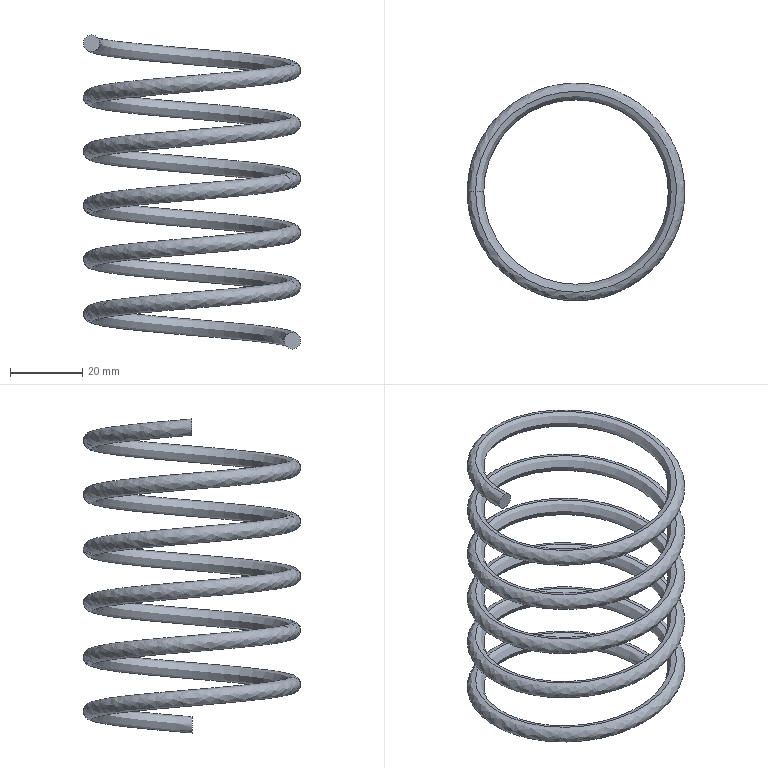Part | SolidWorks | features Helix 1, Sweep 1 | 1 solid | 4 faces | box 60 x 60 x 86.725 mm | volume 15240 mm3 | spline 2 | plane 2